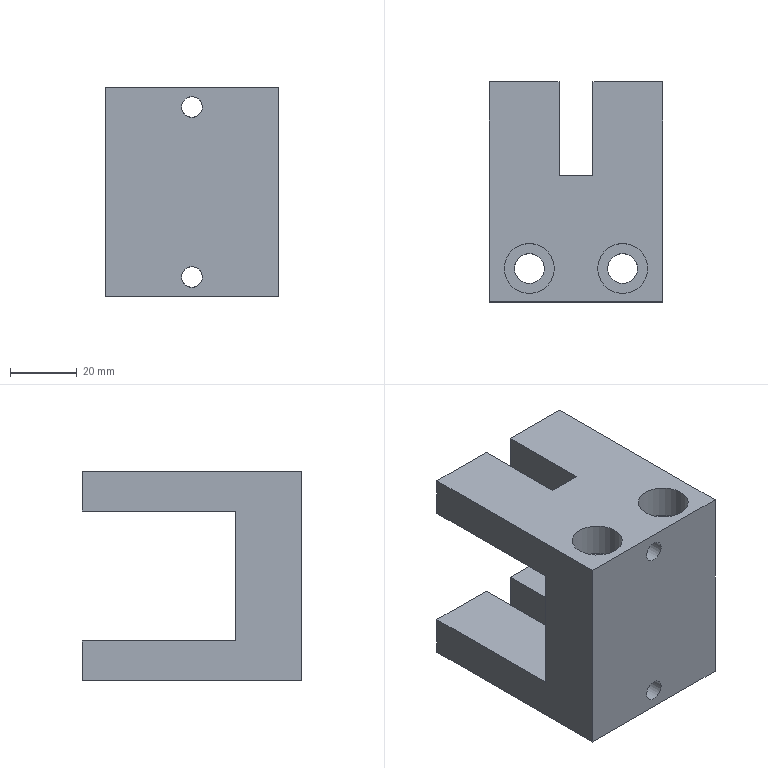CAM job | NX | 3+2 milling, drilling | part box 52 x 66 x 63 mm | stock box 55 x 71 x 65 mm
Tools:
number,name,description,diameter,corner_radius,flute_length,length,flutes
6,D6,平底铣刀-粗,6.0,0.0,25.0,75.0,2
9,D10,平底铣刀-粗,10.0,0.0,35.0,75.0,2
7,D6-J,平底铣刀-精,6.0,0.0,25.0,75.0,2
10,D10-J,平底铣刀-精,10.0,0.0,35.0,75.0,2
1,D80R0.8飞刀,圆鼻刀-粗,80.0,0.8,50.0,75.0,2
2,D6倒角刀,倒角刀,6.0,0.0,3.0,25.0,2
17,ZT6.5,钻头,6.5,0.0,35.0,50.0,2
Operations:
program,operation,operation_type,tool,method,geometry_group,spindle_rpm,surface_speed,feed_per_tooth,feed_cut,feed_plunge,cut_length_mm,path_length_mm,cut_time_min,machine_time_min
A,顶面,FaceMilling,D80R0.8飞刀,侧刃精光-切深K-步距G,W-A,5000.0,1256.637,0.1,1000.0,100.0,157.0,193.0,0.157,0.1606
A,外形粗_2,VolumeBased25DMillingOperation,D10,METHOD,W-A,6000.0,188.496,0.4167,5000.0,80.0,22275.362,22380.162,4.455,4.466
A,底壁粗_1,VolumeBased25DMillingOperation,D10,METHOD,W-A,6000.0,113.0,0.2083,3500.0,100.0,32319.6,34461.647,9.234,9.448
A,底壁粗_2,VolumeBased25DMillingOperation,D6,METHOD,W-A,6000.0,113.0,0.2083,3500.0,100.0,5796.0,6928.232,1.656,1.769
A,打点-深0.8,Operation,D6倒角刀,NONE,W-A,8000.0,150.796,0.0312,500.0,90.0,3.6,155.41,0.0072,0.0224
A,通孔-6-8,Operation,ZT6.5,NONE,W-A,2500.0,48.695,0.06,300.0,90.0,86.0,320.21,0.2867,0.3101
A,底精_1,VolumeBased25DMillingOperation,D10-J,METHOD,W-A,6000.0,113.0,0.2083,1200.0,100.0,407.999,538.999,0.34,0.3531
A,仅选体,SurfaceContour,D6倒角刀,METHOD,W-A,8000.0,150.796,0.1875,3000.0,100.0,332.451,593.35,0.1108,0.1369
A,底侧精_4,VolumeBased25DMillingOperation,D6-J,METHOD,W-A,6000.0,113.0,0.2083,1200.0,100.0,349.906,1559.825,0.2916,0.4126
A,底侧精_3,VolumeBased25DMillingOperation,D10-J,METHOD,W-A,6000.0,188.496,0.0833,1000.0,100.0,784.099,2480.579,0.7841,0.9537
A,外形半精_2,VolumeBased25DMillingOperation,D10-J,METHOD,W-A,6000.0,188.496,0.0833,1000.0,100.0,1065.496,1560.54,1.065,1.115